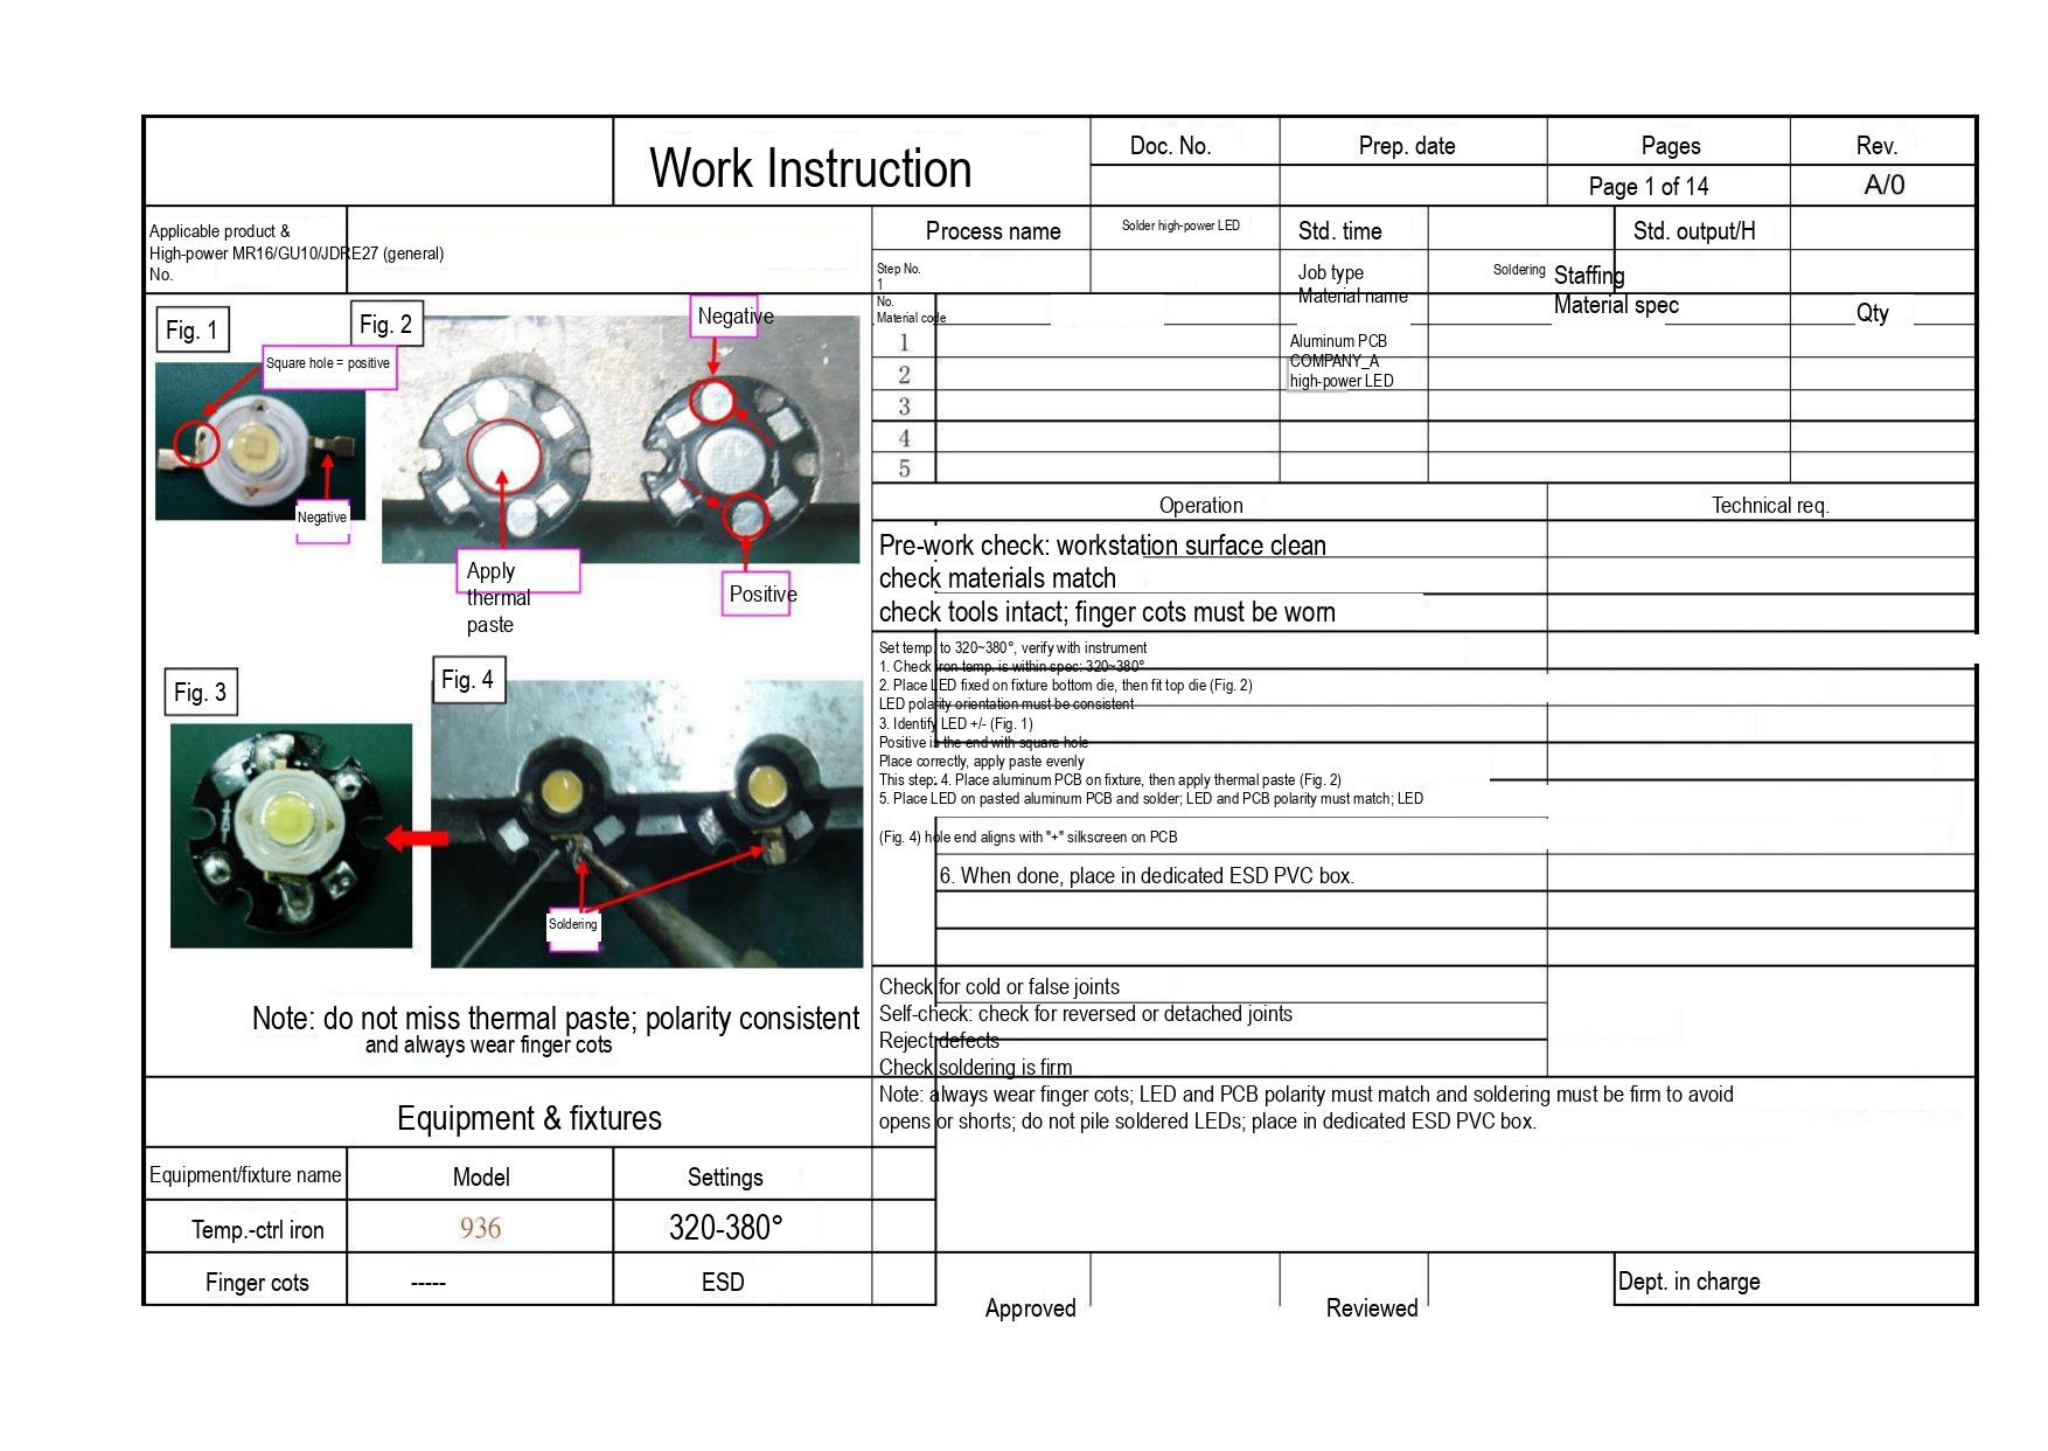# Work Instruction

| Doc. No. | Prep. date | Pages | Rev. |
|---|---|---|---|
| | | Page 1 of 14 | A/0 |

Applicable product &
High-power MR16/GU10/JDRE27 (general)
No.

| Process name | Solder high-power LED | Std. time | | Std. output/H | |
|---|---|---|---|---|---|
| Step No. 1 | | Job type | Soldering | Staffing | |

| No. | Material code | Material name | Material spec | Qty |
|---|---|---|---|---|
| 1 | | Aluminum PCB | | |
| 2 | | COMPANY_A high-power LED | | |
| 3 | | | | |
| 4 | | | | |
| 5 | | | | |

Fig. 1
Square hole = positive
Negative

Fig. 2
Negative
Apply thermal paste
Positive

Fig. 3

Fig. 4
Soldering

Note: do not miss thermal paste; polarity consistent
and always wear finger cots

| Operation | Technical req. |
|---|---|
| Pre-work check: workstation surface clean | |
| check materials match | |
| check tools intact; finger cots must be worn | |
| Set temp to 320~380°, verify with instrument<br>1. Check ~~iron temp. is within spec: 320~380°~~<br>2. Place LED fixed on fixture bottom die, then fit top die (Fig. 2)<br>LED pol~~arity orientation must be consistent~~<br>3. Identify LED +/- (Fig. 1)<br>Positive i~~s the end with square hole~~<br>Place correctly, apply paste evenly<br>This step: 4. Place aluminum PCB on fixture, then apply thermal paste (Fig. 2)<br>5. Place LED on pasted aluminum PCB and solder; LED and PCB polarity must match; LED<br>(Fig. 4) hole end aligns with "+" silkscreen on PCB | |
| 6. When done, place in dedicated ESD PVC box. | |
| Check for cold or false joints<br>Self-check: check for reversed or detached joints<br>Reject ~~defects~~<br>Check soldering is firm | |

Note: always wear finger cots; LED and PCB polarity must match and soldering must be firm to avoid opens or shorts; do not pile soldered LEDs; place in dedicated ESD PVC box.

Equipment & fixtures

| Equipment/fixture name | Model | Settings |
|---|---|---|
| Temp.-ctrl iron | 936 | 320-380° |
| Finger cots | ----- | ESD |

Approved
Reviewed
Dept. in charge
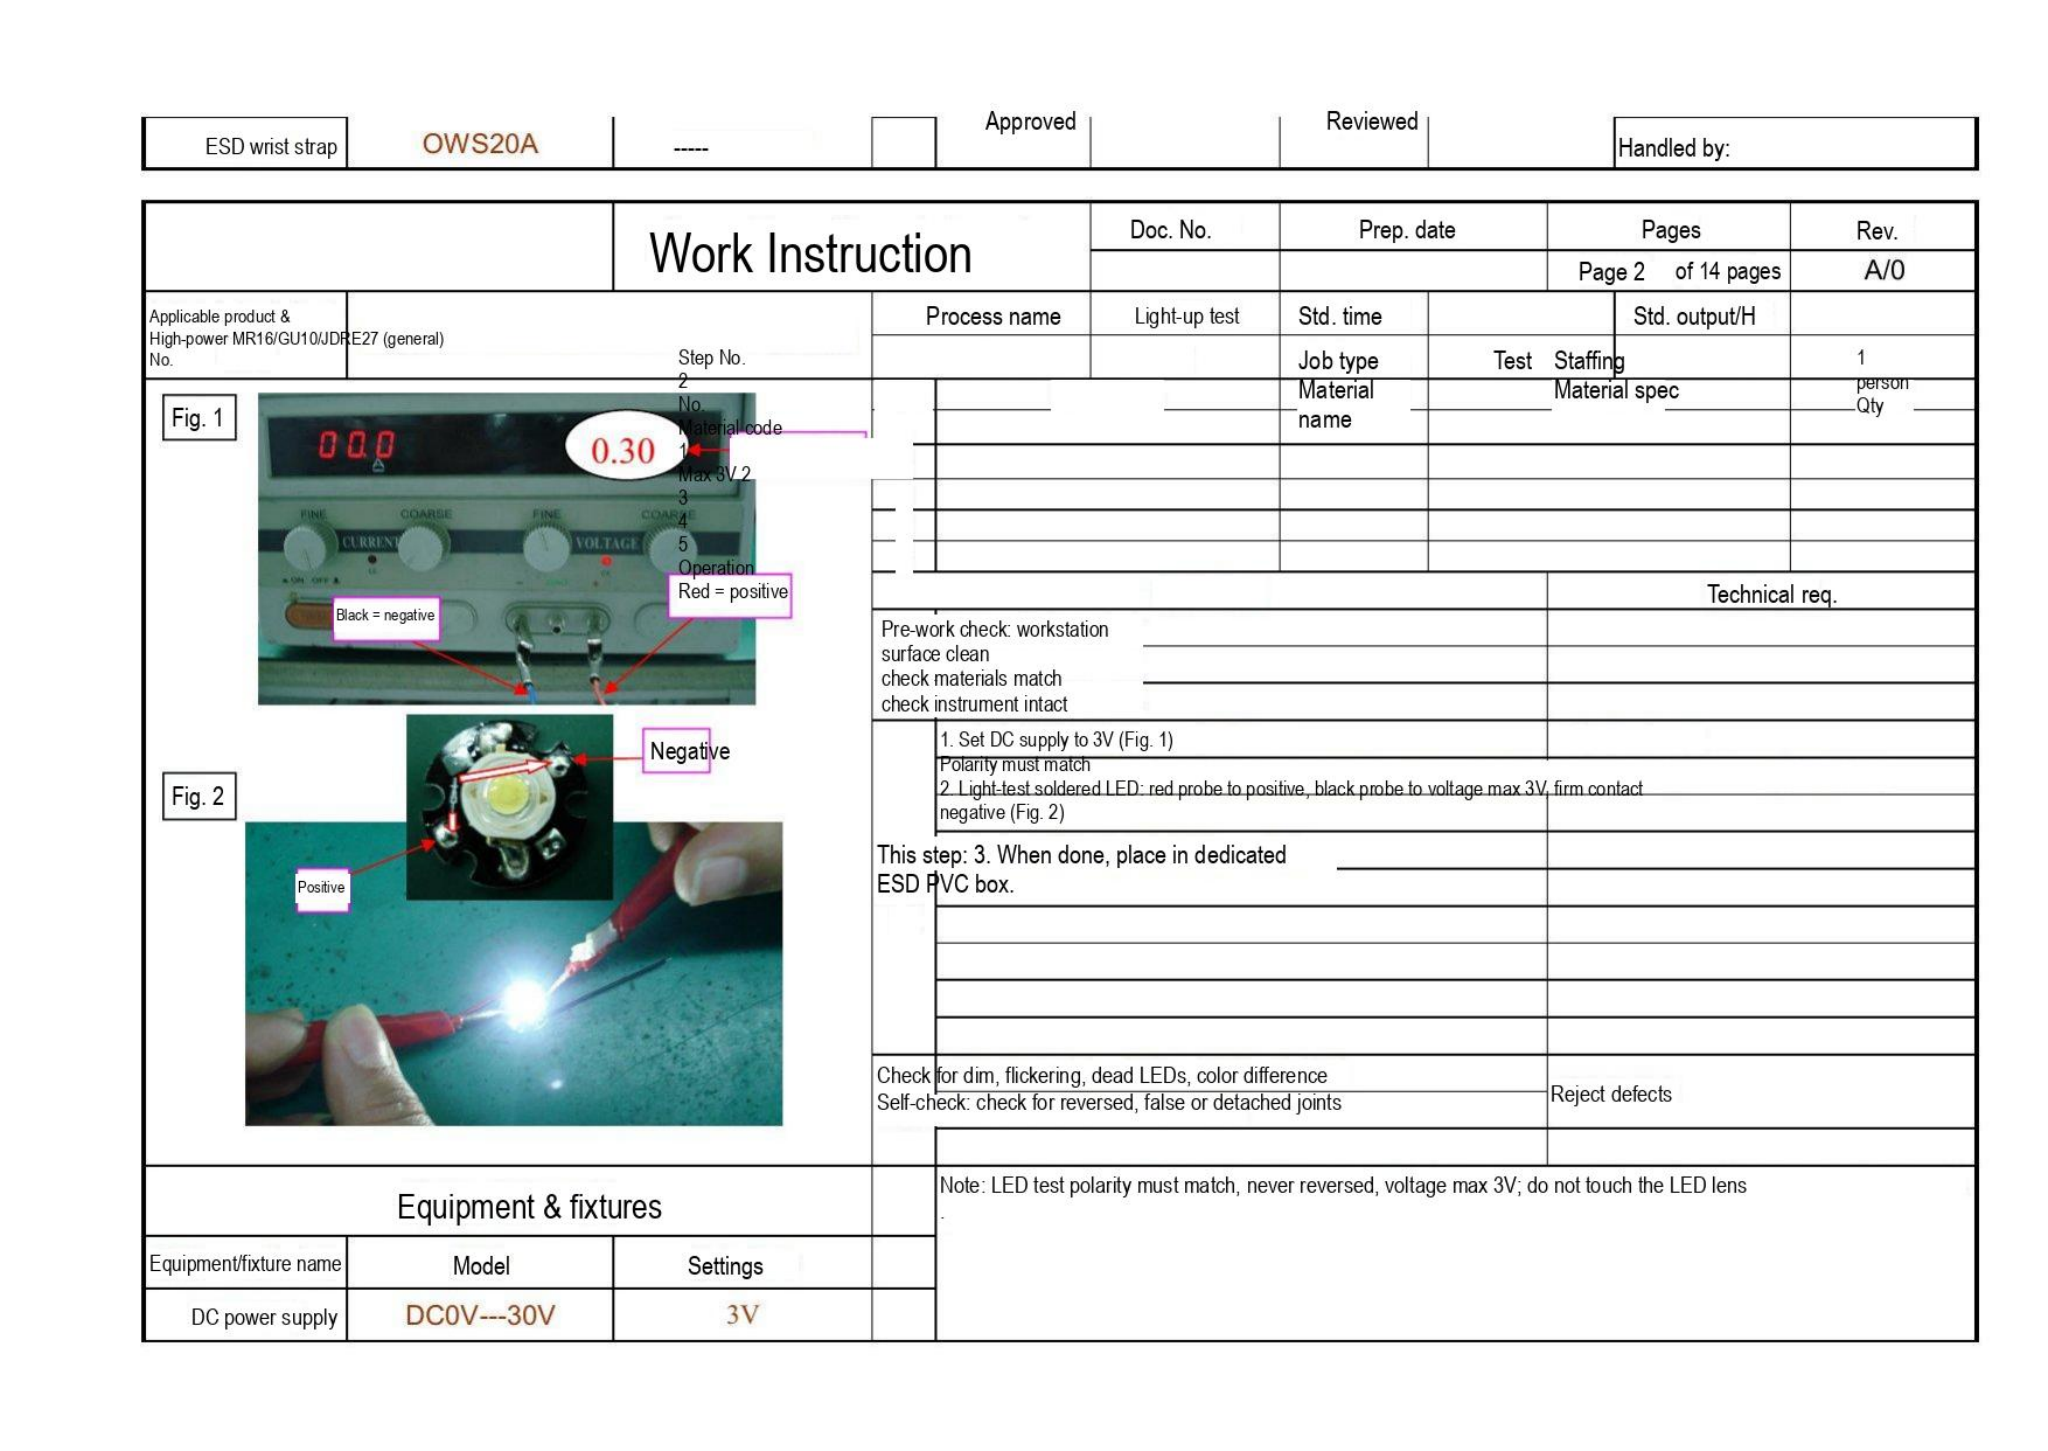| ESD wrist strap | OWS20A | ----- | | Approved | | Reviewed | | Handled by: |
|---|---|---|---|---|---|---|---|---|

| | Work Instruction | Doc. No. | Prep. date | Pages | Rev. |
|---|---|---|---|---|---|
| | | | | Page 2 of 14 pages | A/0 |

| Applicable product & High-power MR16/GU10/JDRE27 (general) No. | Process name | Light-up test | Std. time | | Std. output/H | |
|---|---|---|---|---|---|---|
| | | | Job type | Test | Staffing | 1 person |

Step No. 2
No.
Material code
1
Max 3V 2
3
4
5
Operation

| Material name | Material spec | Qty |
|---|---|---|
| | | |
| | | |
| | | |
| | | |

Fig. 1

0 0.0

0.30

FINE COARSE FINE COARSE
CURRENT VOLTAGE
ON OFF

Black = negative

Red = positive

Fig. 2

Negative

Positive

| Operation | Technical req. |
|---|---|
| Pre-work check: workstation surface clean<br>check materials match<br>check instrument intact | |
| 1. Set DC supply to 3V (Fig. 1)<br>Polarity must match | |
| 2. Light-test soldered LED: red probe to positive, black probe to voltage max 3V, firm contact negative (Fig. 2) | |
| This step: 3. When done, place in dedicated ESD PVC box. | |
| Check for dim, flickering, dead LEDs, color difference<br>Self-check: check for reversed, false or detached joints | Reject defects |

Note: LED test polarity must match, never reversed, voltage max 3V; do not touch the LED lens

Equipment & fixtures

| Equipment/fixture name | Model | Settings |
|---|---|---|
| DC power supply | DC0V---30V | 3V |
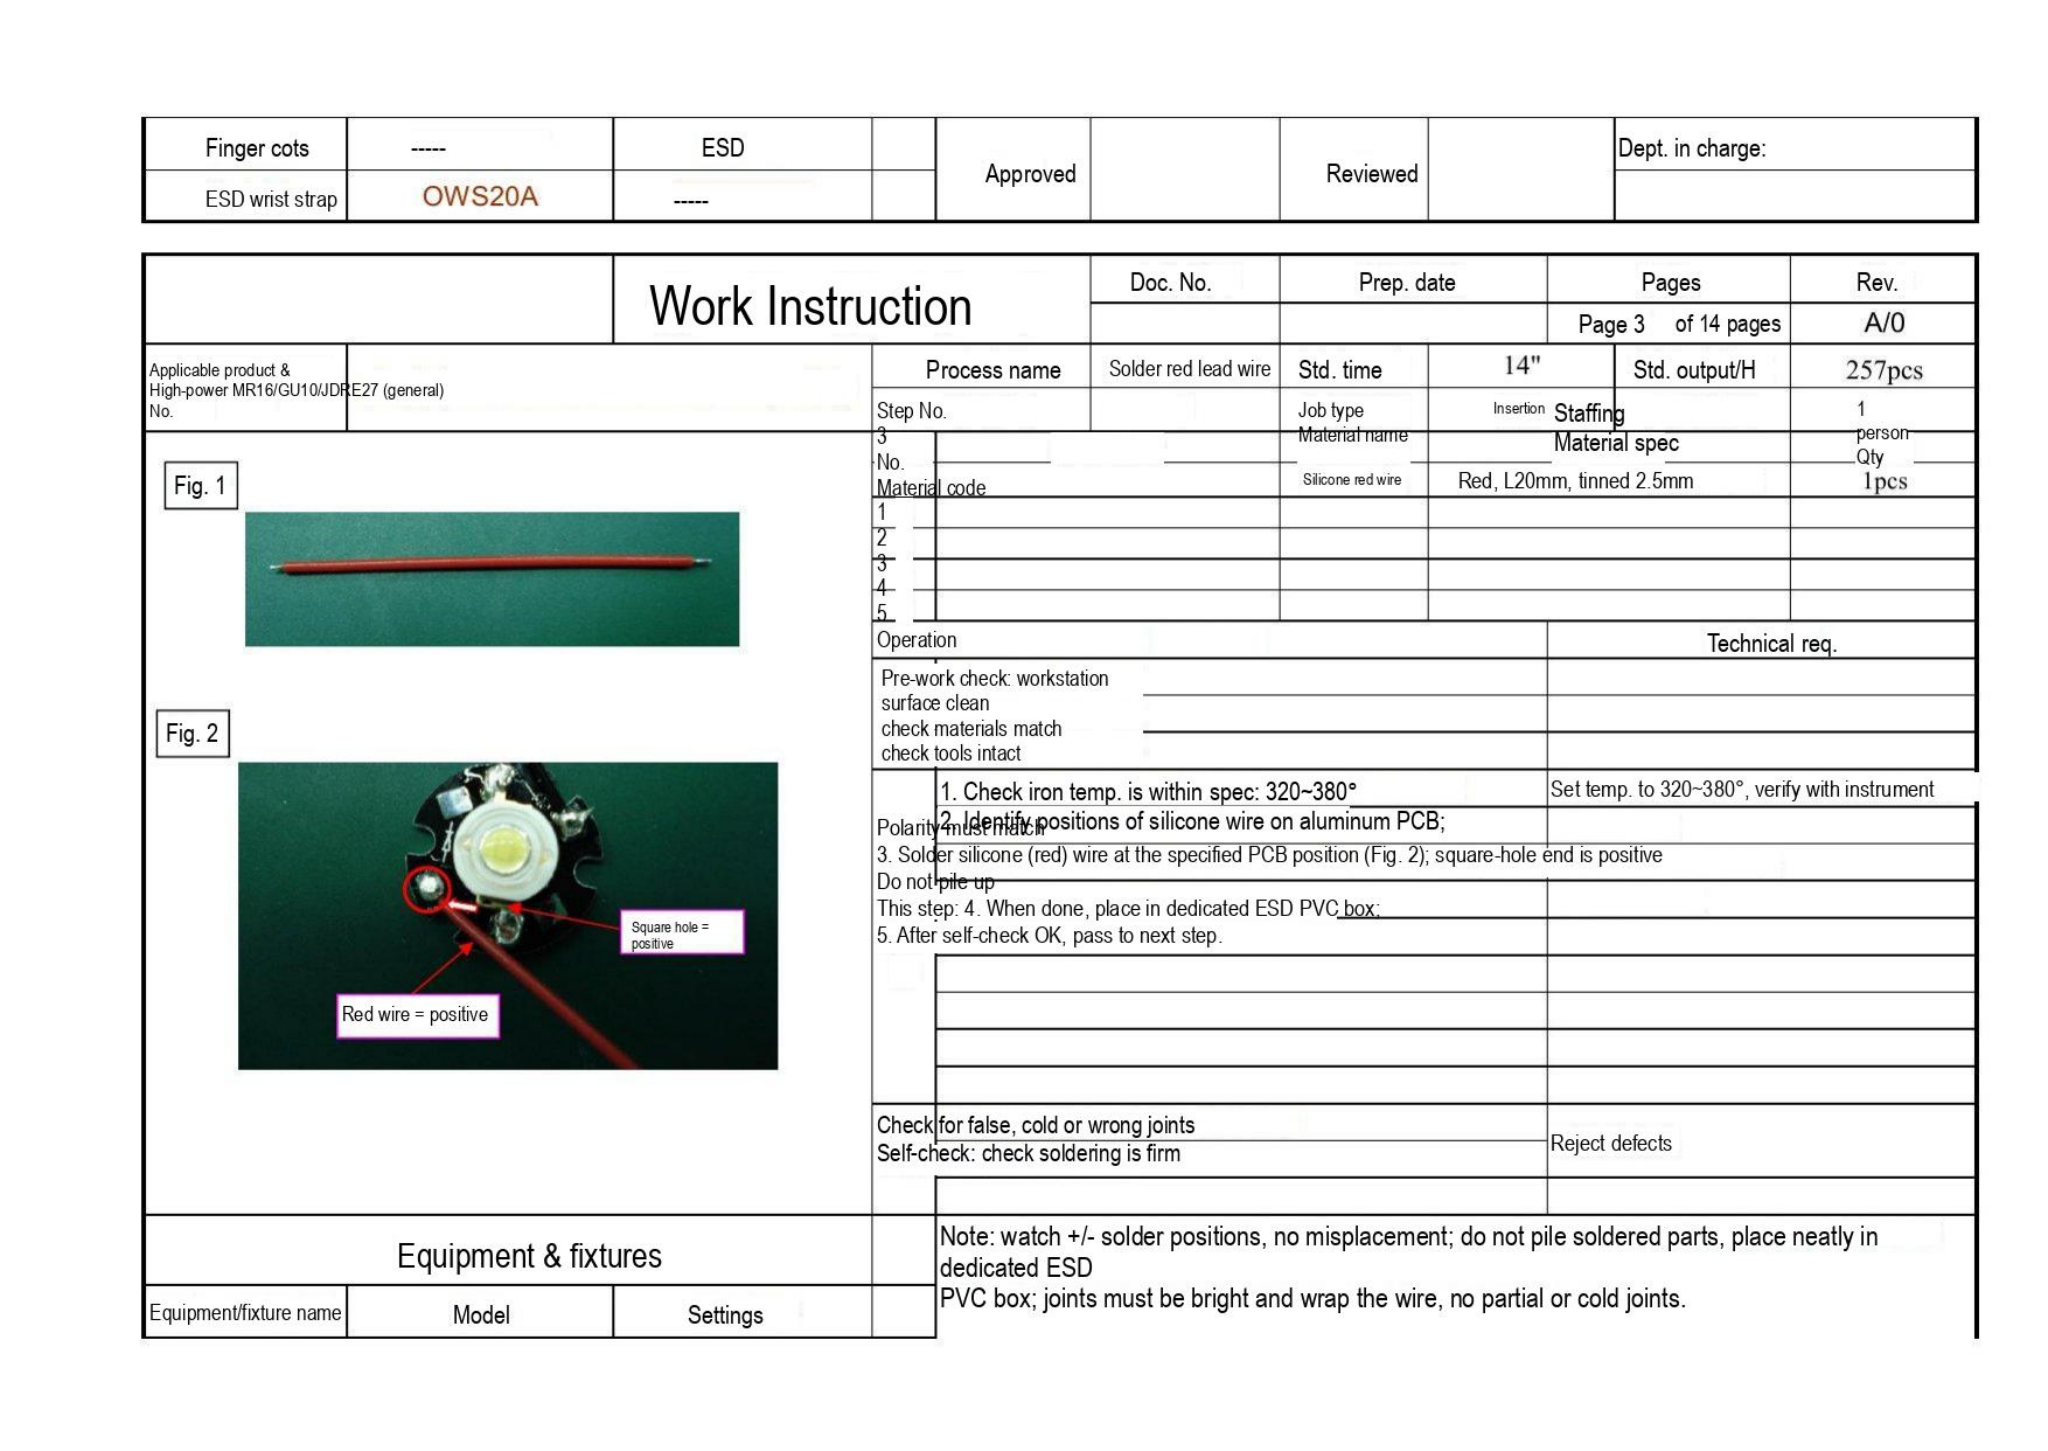| Finger cots | ----- | ESD | | Approved | | Reviewed | | Dept. in charge: |
|---|---|---|---|---|---|---|---|---|
| ESD wrist strap | OWS20A | ----- | | | | | | |

| Work Instruction | Doc. No. | Prep. date | Pages | Rev. |
|---|---|---|---|---|
| | | | Page 3 of 14 pages | A/0 |

| Applicable product & High-power MR16/GU10/JDRE27 (general) No. | Process name | Solder red lead wire | Std. time | 14" | Std. output/H | 257pcs |
|---|---|---|---|---|---|---|
| | Step No. 3 | | Job type | Insertion | Staffing | 1 person |

| No. | Material code | Material name | Material spec | Qty |
|---|---|---|---|---|
| | | Silicone red wire | Red, L20mm, tinned 2.5mm | 1pcs |
| 1 | | | | |
| 2 | | | | |
| 3 | | | | |
| 4 | | | | |
| 5 | | | | |

Fig. 1

Fig. 2

Square hole = positive

Red wire = positive

| Operation | Technical req. |
|---|---|
| Pre-work check: workstation surface clean<br>check materials match<br>check tools intact | |
| 1. Check iron temp. is within spec: 320~380° | Set temp. to 320~380°, verify with instrument |
| Polarity must match 2. Identify positions of silicone wire on aluminum PCB; | |
| 3. Solder silicone (red) wire at the specified PCB position (Fig. 2); square-hole end is positive<br>Do not pile up | |
| This step: 4. When done, place in dedicated ESD PVC box; | |
| 5. After self-check OK, pass to next step. | |
| Check for false, cold or wrong joints<br>Self-check: check soldering is firm | Reject defects |

Note: watch +/- solder positions, no misplacement; do not pile soldered parts, place neatly in dedicated ESD PVC box; joints must be bright and wrap the wire, no partial or cold joints.

| Equipment & fixtures | | |
|---|---|---|
| Equipment/fixture name | Model | Settings |
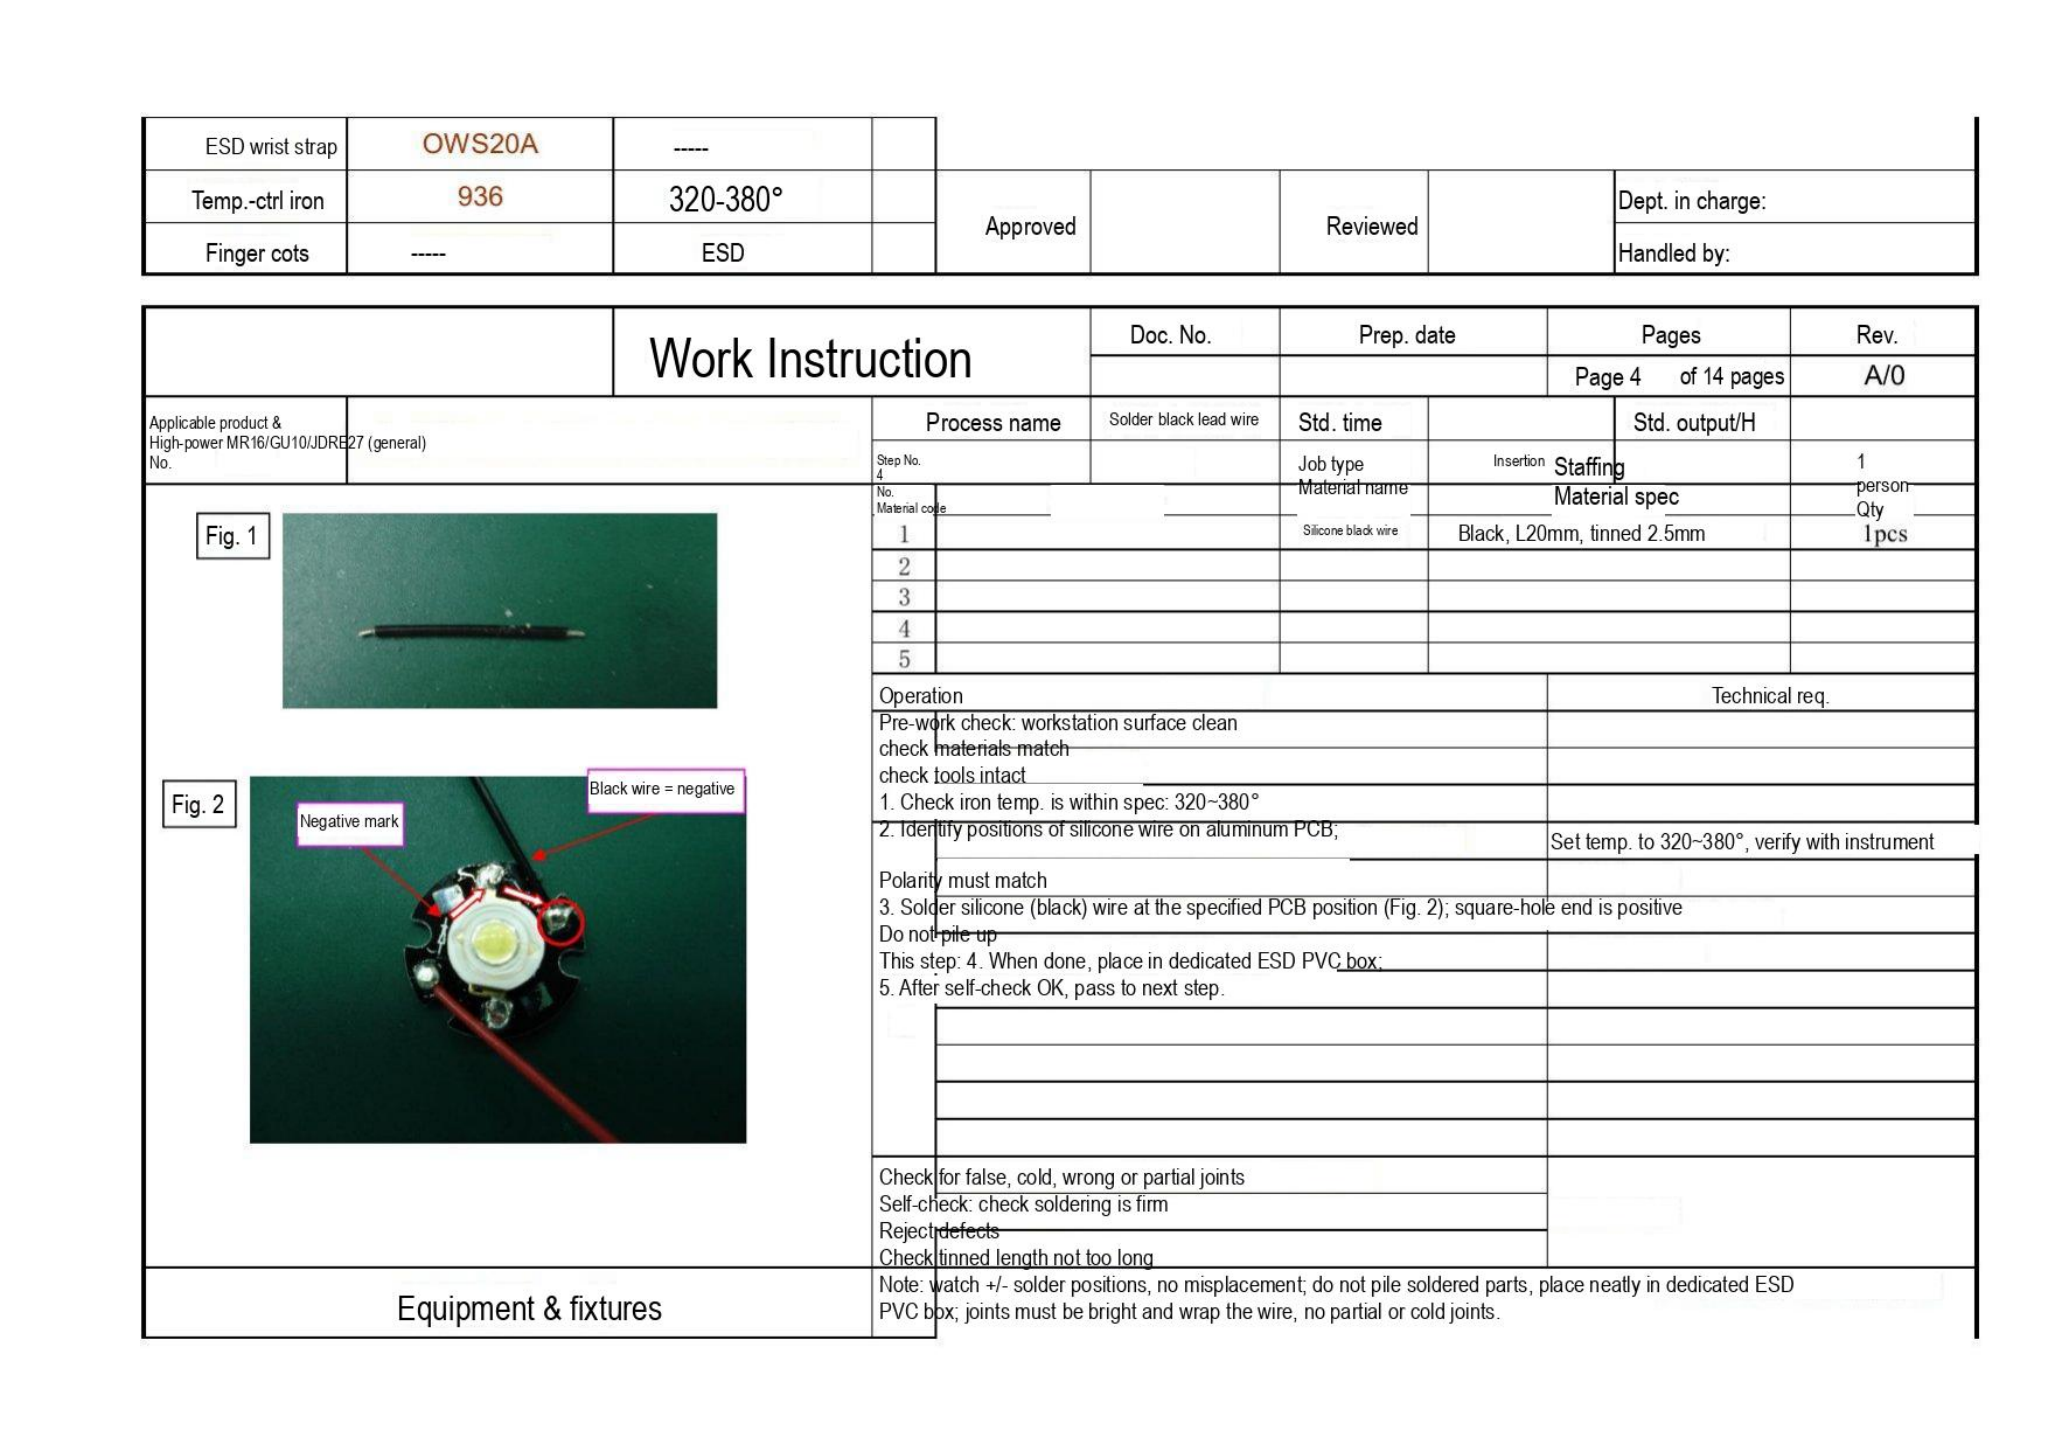| ESD wrist strap | OWS20A | ----- | |
|---|---|---|---|
| Temp.-ctrl iron | 936 | 320-380° | |
| Finger cots | ----- | ESD | |

| Approved | | Reviewed | | Dept. in charge: |
|---|---|---|---|---|
| | | | | Handled by: |

| | Work Instruction | Doc. No. | Prep. date | Pages | Rev. |
|---|---|---|---|---|---|
| | | | | Page 4 of 14 pages | A/0 |

| Applicable product & No. | Process name | Solder black lead wire | Std. time | | Std. output/H | |
|---|---|---|---|---|---|---|
| High-power MR16/GU10/JDRE27 (general) | Step No. 4 | | Job type | Insertion | Staffing | 1 person |

| No. | Material code | Material name | Material spec | Qty |
|---|---|---|---|---|
| 1 | | Silicone black wire | Black, L20mm, tinned 2.5mm | 1pcs |
| 2 | | | | |
| 3 | | | | |
| 4 | | | | |
| 5 | | | | |

Fig. 1

Fig. 2

Negative mark

Black wire = negative

| Operation | Technical req. |
|---|---|
| Pre-work check: workstation surface clean | |
| check materials match | |
| check tools intact | |
| 1. Check iron temp. is within spec: 320~380° | |
| 2. Identify positions of silicone wire on aluminum PCB; | Set temp. to 320~380°, verify with instrument |
| Polarity must match | |
| 3. Solder silicone (black) wire at the specified PCB position (Fig. 2); square-hole end is positive | |
| Do not pile up | |
| This step: 4. When done, place in dedicated ESD PVC box; | |
| 5. After self-check OK, pass to next step. | |
| | |
| | |
| | |
| | |
| Check for false, cold, wrong or partial joints | |
| Self-check: check soldering is firm | |
| Reject defects | |
| Check tinned length not too long | |

| Equipment & fixtures | Note: watch +/- solder positions, no misplacement; do not pile soldered parts, place neatly in dedicated ESD PVC box; joints must be bright and wrap the wire, no partial or cold joints. |
|---|---|
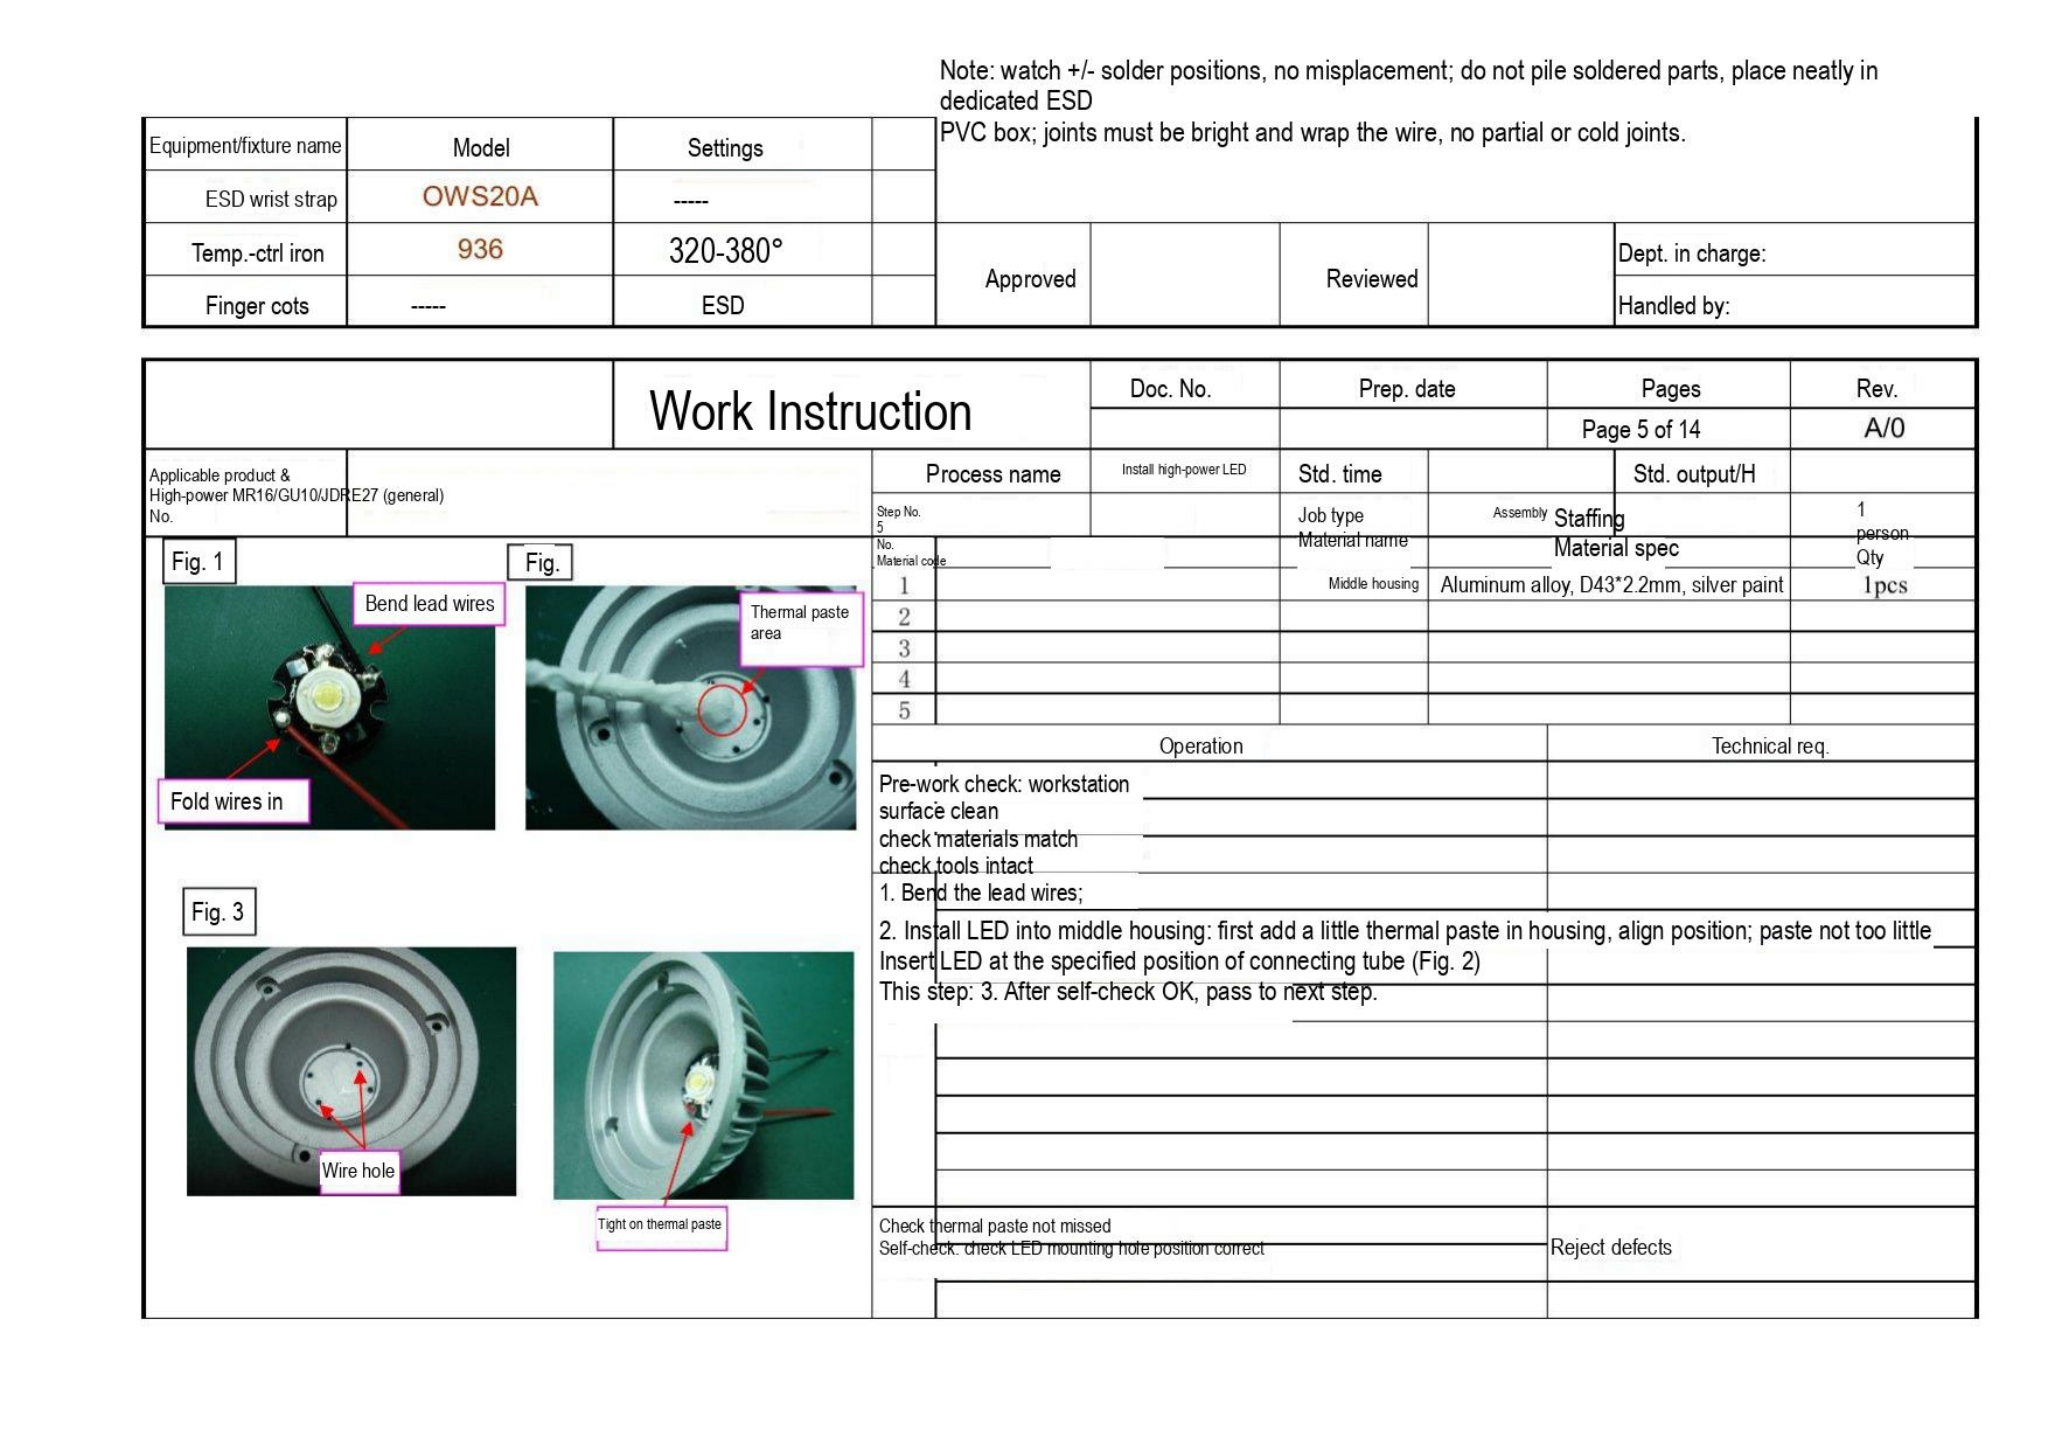Note: watch +/- solder positions, no misplacement; do not pile soldered parts, place neatly in dedicated ESD
PVC box; joints must be bright and wrap the wire, no partial or cold joints.

| Equipment/fixture name | Model | Settings | |
|---|---|---|---|
| ESD wrist strap | OWS20A | ----- | |
| Temp.-ctrl iron | 936 | 320-380° | |
| Finger cots | ----- | ESD | |

| Approved | | Reviewed | | Dept. in charge: |
|---|---|---|---|---|
| | | | | Handled by: |

| | Work Instruction | Doc. No. | Prep. date | Pages | Rev. |
|---|---|---|---|---|---|
| | | | | Page 5 of 14 | A/0 |

| Applicable product & No. | High-power MR16/GU10/JDRE27 (general) |
|---|---|

| Process name | Install high-power LED | Std. time | | Std. output/H | |
|---|---|---|---|---|---|
| Step No. 5 | | Job type | Assembly | Staffing | 1 person |
| No. | Material code | Material name | Material spec | | Qty |
| 1 | | Middle housing | Aluminum alloy, D43*2.2mm, silver paint | | 1pcs |
| 2 | | | | | |
| 3 | | | | | |
| 4 | | | | | |
| 5 | | | | | |

Fig. 1
Bend lead wires
Fold wires in

Fig.
Thermal paste area

Fig. 3
Wire hole
Tight on thermal paste

| Operation | Technical req. |
|---|---|
| Pre-work check: workstation surface clean<br>check materials match<br>check tools intact | |
| 1. Bend the lead wires; | |
| 2. Install LED into middle housing: first add a little thermal paste in housing, align position; paste not too little<br>Insert LED at the specified position of connecting tube (Fig. 2)<br>This step: 3. After self-check OK, pass to next step. | |
| | |
| | |
| | |
| | |
| Check thermal paste not missed<br>Self-check: check LED mounting hole position correct | Reject defects |
| | |
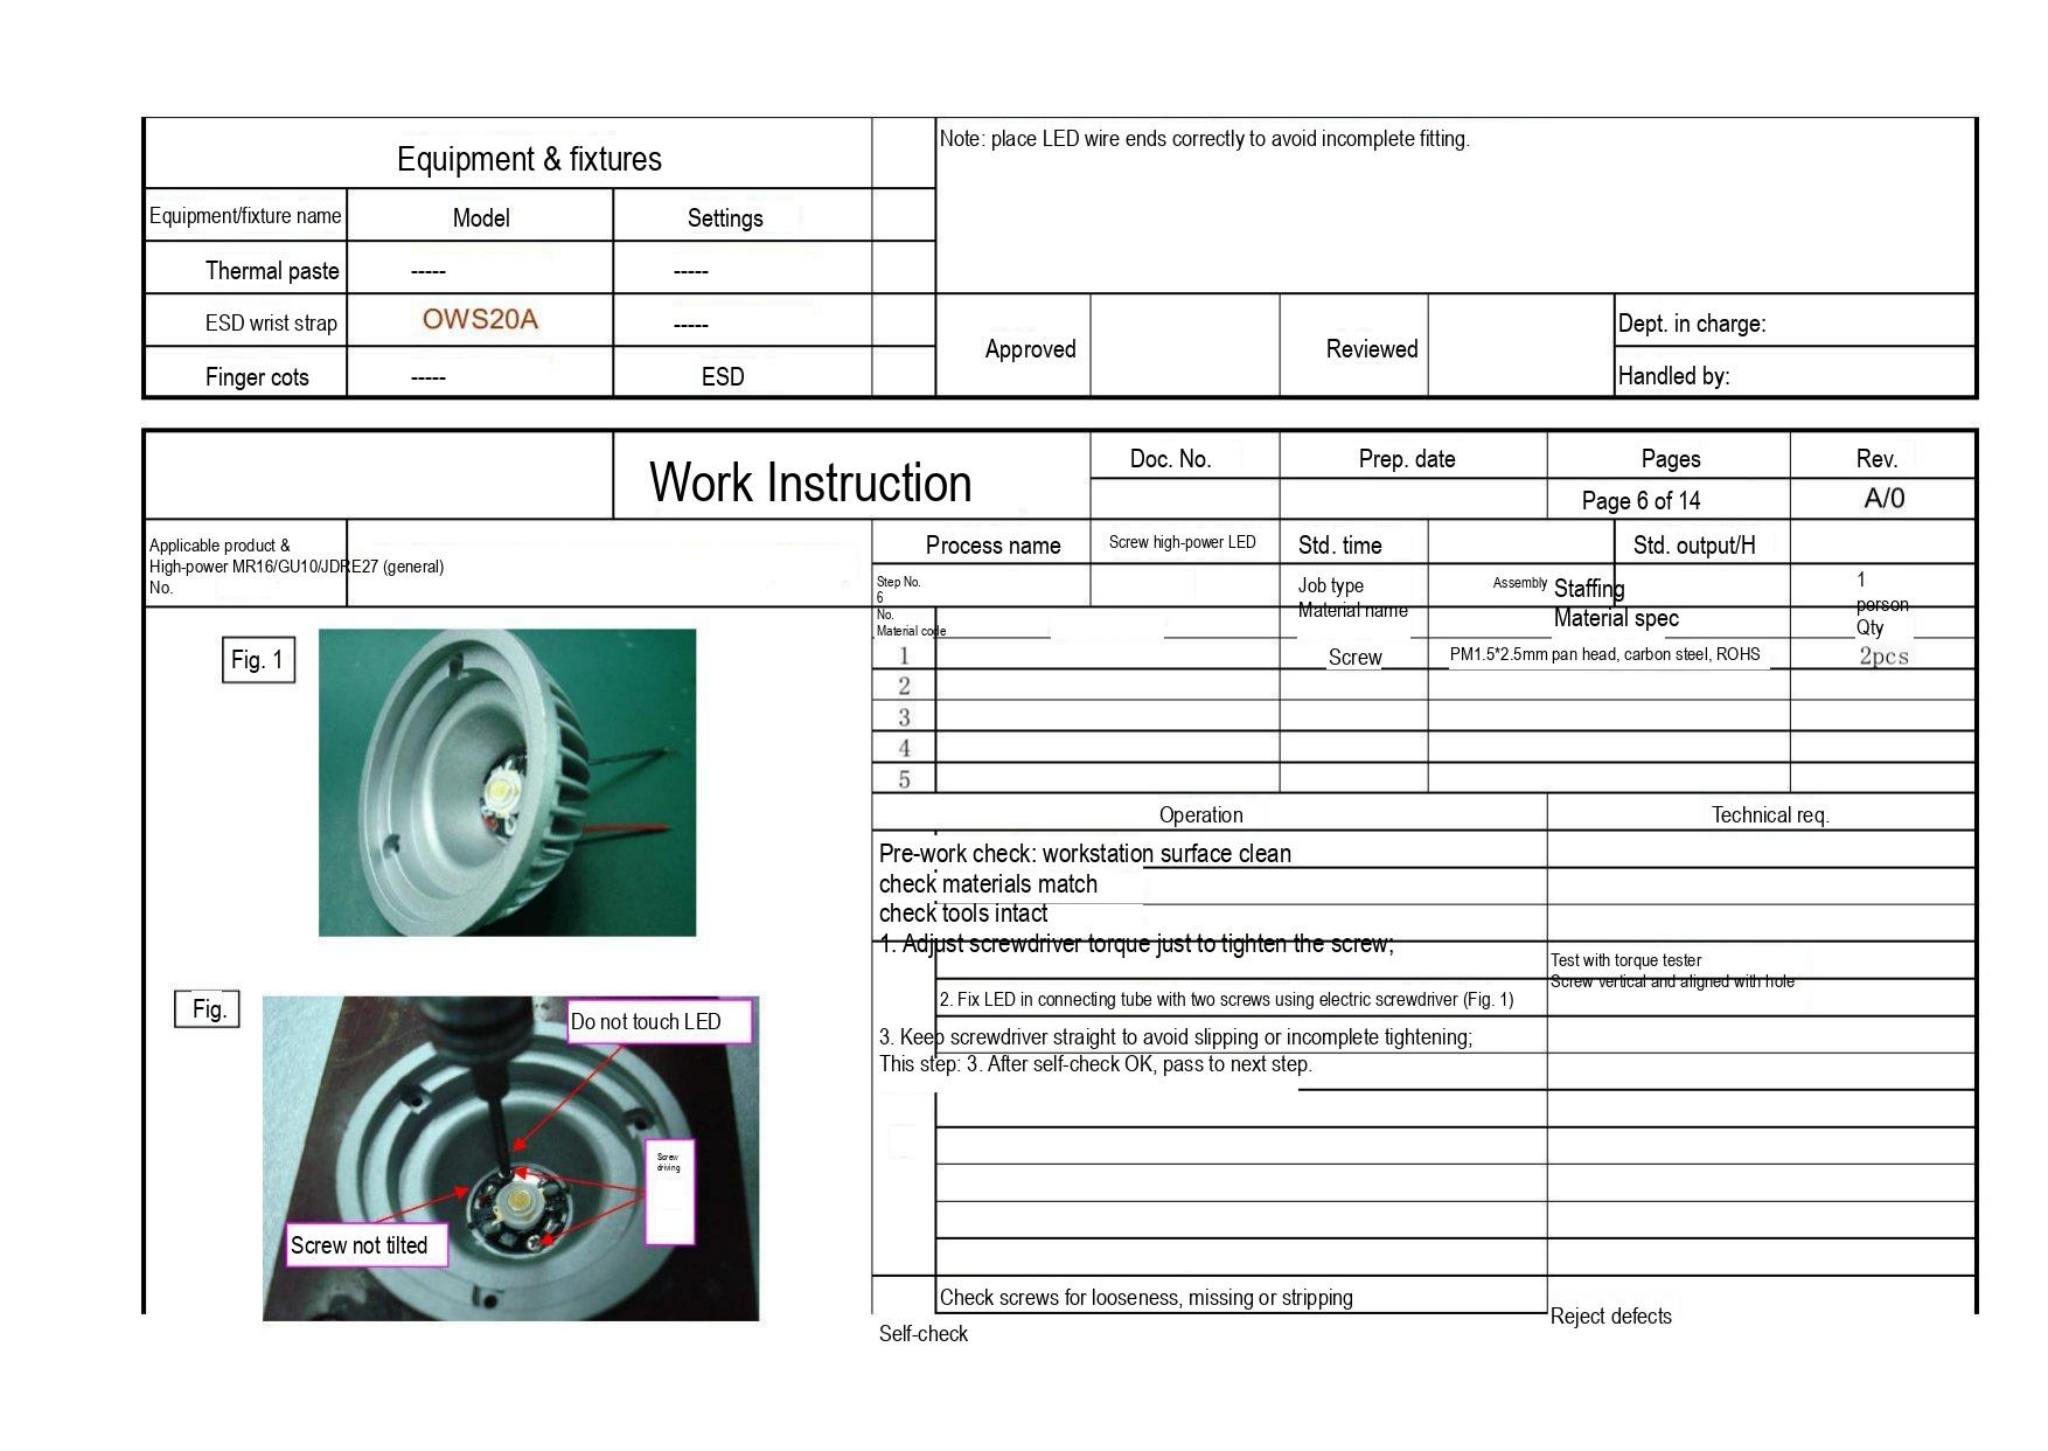| Equipment & fixtures | | |
|---|---|---|
| Equipment/fixture name | Model | Settings |
| Thermal paste | ----- | ----- |
| ESD wrist strap | OWS20A | ----- |
| Finger cots | ----- | ESD |

Note: place LED wire ends correctly to avoid incomplete fitting.

| Approved | | Reviewed | | Dept. in charge: |
|---|---|---|---|---|
| | | | | Handled by: |

| Work Instruction | Doc. No. | Prep. date | Pages | Rev. |
|---|---|---|---|---|
| | | | Page 6 of 14 | A/0 |

Applicable product & No.: High-power MR16/GU10/JDRE27 (general)

| Process name | Screw high-power LED | Std. time | | Std. output/H | |
|---|---|---|---|---|---|
| Step No. 6 | | Job type | Assembly | Staffing | 1 person |

| No. | Material code | Material name | Material spec | Qty |
|---|---|---|---|---|
| 1 | | Screw | PM1.5*2.5mm pan head, carbon steel, ROHS | 2pcs |
| 2 | | | | |
| 3 | | | | |
| 4 | | | | |
| 5 | | | | |

Fig. 1

Fig.

Do not touch LED

Screw driving

Screw not tilted

| Operation | Technical req. |
|---|---|
| Pre-work check: workstation surface clean<br>check materials match<br>check tools intact | |
| 1. Adjust screwdriver torque just to tighten the screw; | Test with torque tester |
| 2. Fix LED in connecting tube with two screws using electric screwdriver (Fig. 1) | Screw vertical and aligned with hole |
| 3. Keep screwdriver straight to avoid slipping or incomplete tightening;<br>This step: 3. After self-check OK, pass to next step. | |
| Self-check: Check screws for looseness, missing or stripping | Reject defects |